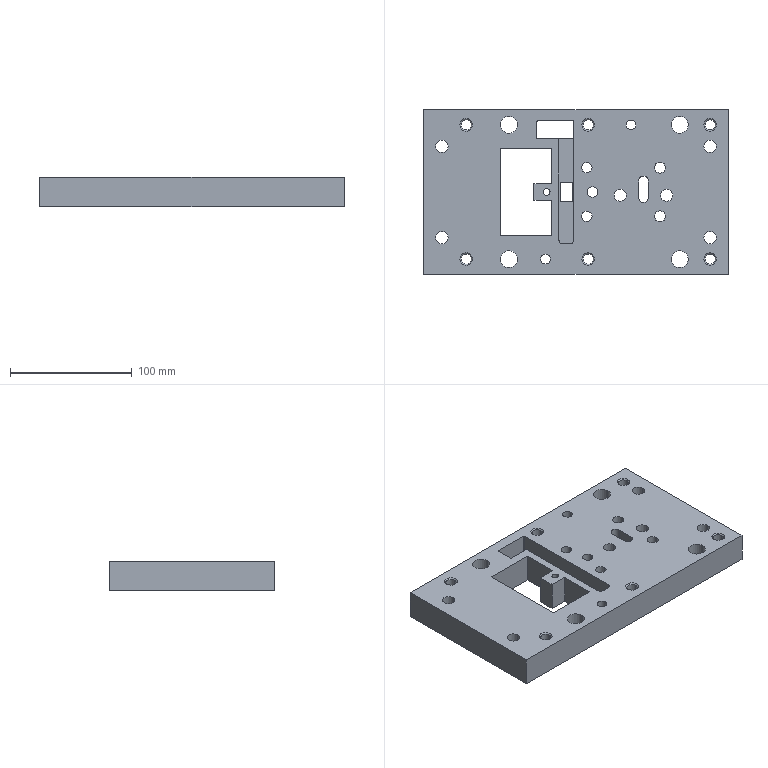Part | STEP file | MIENG TRUNG GIAN DUOI | 1 solid | 133 faces | box 250 x 135 x 24 mm | volume 656672 mm3 | cylinder 72 | plane 33 | cone 28 | commonest cylinder face diameters 8.376 x16 14 x14 10.106 x8 8 x6 8.5 x6 10 x6